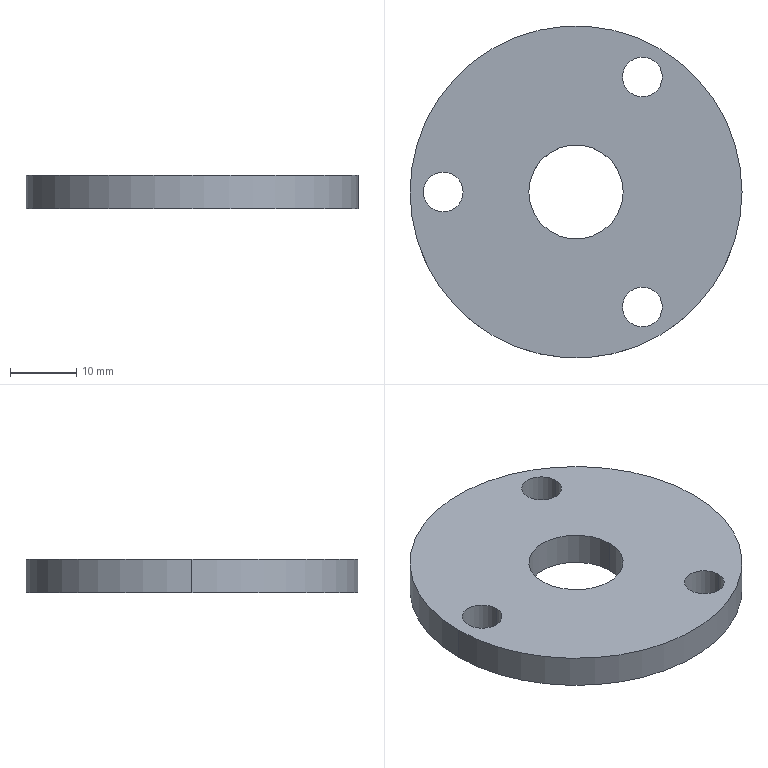Part | STEP file | 1 solid | 12 faces | box 50 x 50 x 5 mm | volume 8602 mm3 | cylinder 10 | plane 2 | commonest cylinder face diameters 6 x6 14.2 x2 50 x2
STEP:
#1=CARTESIAN_POINT('',(0.,0.,0.));
#2=DIRECTION('',(0.,0.,1.));
#3=DIRECTION('',(1.,0.,0.));
#4=AXIS2_PLACEMENT_3D('',#1,#2,#3);
#5=CARTESIAN_POINT('',(13.,17.321,0.));
#6=VERTEX_POINT('',#5);
#7=CARTESIAN_POINT('',(13.,17.321,5.));
#8=VERTEX_POINT('',#7);
#9=CARTESIAN_POINT('',(13.,17.321,15.));
#10=DIRECTION('',(0.,0.,1.));
#11=VECTOR('',#10,1.);
#12=LINE('',#9,#11);
#13=CARTESIAN_POINT('',(10.,17.321,15.));
#14=DIRECTION('',(0.,0.,1.));
#15=DIRECTION('',(1.,0.,0.));
#16=AXIS2_PLACEMENT_3D('',#13,#14,#15);
#17=CYLINDRICAL_SURFACE('',#16,3.);
#18=CARTESIAN_POINT('',(6.283,0.));
#19=DIRECTION('',(0.,1.));
#20=VECTOR('',#19,1.);
#21=LINE('',#18,#20);
#22=(GEOMETRIC_REPRESENTATION_CONTEXT(2)PARAMETRIC_REPRESENTATION_CONTEXT()REPRESENTATION_CONTEXT('',''));
#23=DEFINITIONAL_REPRESENTATION('',(#21),#22);
#24=PCURVE('',#17,#23);
#25=CARTESIAN_POINT('',(10.,17.321,15.));
#26=DIRECTION('',(0.,0.,1.));
#27=DIRECTION('',(1.,0.,0.));
#28=AXIS2_PLACEMENT_3D('',#25,#26,#27);
#29=CYLINDRICAL_SURFACE('',#28,3.);
#30=CARTESIAN_POINT('',(0.,0.));
#31=DIRECTION('',(0.,1.));
#32=VECTOR('',#31,1.);
#33=LINE('',#30,#32);
#34=(GEOMETRIC_REPRESENTATION_CONTEXT(2)PARAMETRIC_REPRESENTATION_CONTEXT()REPRESENTATION_CONTEXT('',''));
#35=DEFINITIONAL_REPRESENTATION('',(#33),#34);
#36=PCURVE('',#29,#35);
#37=SURFACE_CURVE('',#12,(#24,#36),.PCURVE_S1.);
#38=EDGE_CURVE('',#6,#8,#37,.T.);
#39=ORIENTED_EDGE('',*,*,#38,.T.);
#40=CARTESIAN_POINT('',(7.,17.321,5.));
#41=VERTEX_POINT('',#40);
#42=CARTESIAN_POINT('',(10.,17.321,5.));
#43=DIRECTION('',(0.,0.,-1.));
#44=DIRECTION('',(1.,0.,0.));
#45=AXIS2_PLACEMENT_3D('',#42,#43,#44);
#46=CIRCLE('',#45,3.);
#47=CARTESIAN_POINT('',(6.283,-10.));
#48=DIRECTION('',(-1.,0.));
#49=VECTOR('',#48,1.);
#50=LINE('',#47,#49);
#51=(GEOMETRIC_REPRESENTATION_CONTEXT(2)PARAMETRIC_REPRESENTATION_CONTEXT()REPRESENTATION_CONTEXT('',''));
#52=DEFINITIONAL_REPRESENTATION('',(#50),#51);
#53=PCURVE('',#17,#52);
#54=CARTESIAN_POINT('',(0.,0.,5.));
#55=DIRECTION('',(0.,0.,1.));
#56=DIRECTION('',(1.,0.,0.));
#57=AXIS2_PLACEMENT_3D('',#54,#55,#56);
#58=PLANE('',#57);
#59=CARTESIAN_POINT('',(13.,17.321));
#60=CARTESIAN_POINT('',(13.,12.124));
#61=CARTESIAN_POINT('',(8.5,14.722));
#62=CARTESIAN_POINT('',(4.,17.321));
#63=CARTESIAN_POINT('',(8.5,19.919));
#64=CARTESIAN_POINT('',(13.,22.517));
#65=CARTESIAN_POINT('',(13.,17.321));
#66=(BOUNDED_CURVE()B_SPLINE_CURVE(2,(#59,#60,#61,#62,#63,#64,#65),.UNSPECIFIED.,.T.,.F.)B_SPLINE_CURVE_WITH_KNOTS((1,2,2,2,2,1),(-2.094,0.,2.094,4.189,6.283,8.378),.UNSPECIFIED.)CURVE()GEOMETRIC_REPRESENTATION_ITEM()RATIONAL_B_SPLINE_CURVE((1.,0.5,1.,0.5,1.,0.5,1.))REPRESENTATION_ITEM(''));
#67=(GEOMETRIC_REPRESENTATION_CONTEXT(2)PARAMETRIC_REPRESENTATION_CONTEXT()REPRESENTATION_CONTEXT('',''));
#68=DEFINITIONAL_REPRESENTATION('',(#66),#67);
#69=PCURVE('',#58,#68);
#70=SURFACE_CURVE('',#46,(#53,#69),.PCURVE_S1.);
#71=EDGE_CURVE('',#8,#41,#70,.T.);
#72=ORIENTED_EDGE('',*,*,#71,.T.);
#73=CARTESIAN_POINT('',(7.,17.321,0.));
#74=VERTEX_POINT('',#73);
#75=CARTESIAN_POINT('',(7.,17.321,15.));
#76=DIRECTION('',(0.,0.,1.));
#77=VECTOR('',#76,1.);
#78=LINE('',#75,#77);
#79=CARTESIAN_POINT('',(3.142,0.));
#80=DIRECTION('',(0.,1.));
#81=VECTOR('',#80,1.);
#82=LINE('',#79,#81);
#83=(GEOMETRIC_REPRESENTATION_CONTEXT(2)PARAMETRIC_REPRESENTATION_CONTEXT()REPRESENTATION_CONTEXT('',''));
#84=DEFINITIONAL_REPRESENTATION('',(#82),#83);
#85=PCURVE('',#17,#84);
#86=CARTESIAN_POINT('',(3.142,0.));
#87=DIRECTION('',(0.,1.));
#88=VECTOR('',#87,1.);
#89=LINE('',#86,#88);
#90=(GEOMETRIC_REPRESENTATION_CONTEXT(2)PARAMETRIC_REPRESENTATION_CONTEXT()REPRESENTATION_CONTEXT('',''));
#91=DEFINITIONAL_REPRESENTATION('',(#89),#90);
#92=PCURVE('',#29,#91);
#93=SURFACE_CURVE('',#78,(#85,#92),.PCURVE_S1.);
#94=EDGE_CURVE('',#74,#41,#93,.T.);
#95=ORIENTED_EDGE('',*,*,#94,.F.);
#96=CARTESIAN_POINT('',(10.,17.321,0.));
#97=DIRECTION('',(0.,0.,1.));
#98=DIRECTION('',(1.,0.,0.));
#99=AXIS2_PLACEMENT_3D('',#96,#97,#98);
#100=CIRCLE('',#99,3.);
#101=CARTESIAN_POINT('',(0.,-15.));
#102=DIRECTION('',(1.,0.));
#103=VECTOR('',#102,1.);
#104=LINE('',#101,#103);
#105=(GEOMETRIC_REPRESENTATION_CONTEXT(2)PARAMETRIC_REPRESENTATION_CONTEXT()REPRESENTATION_CONTEXT('',''));
#106=DEFINITIONAL_REPRESENTATION('',(#104),#105);
#107=PCURVE('',#17,#106);
#108=CARTESIAN_POINT('',(0.,0.,0.));
#109=DIRECTION('',(0.,0.,1.));
#110=DIRECTION('',(1.,0.,0.));
#111=AXIS2_PLACEMENT_3D('',#108,#109,#110);
#112=PLANE('',#111);
#113=CARTESIAN_POINT('',(10.,17.321));
#114=DIRECTION('',(1.,0.));
#115=AXIS2_PLACEMENT_2D('',#113,#114);
#116=CIRCLE('',#115,3.);
#117=(GEOMETRIC_REPRESENTATION_CONTEXT(2)PARAMETRIC_REPRESENTATION_CONTEXT()REPRESENTATION_CONTEXT('',''));
#118=DEFINITIONAL_REPRESENTATION('',(#116),#117);
#119=PCURVE('',#112,#118);
#120=SURFACE_CURVE('',#100,(#107,#119),.PCURVE_S1.);
#121=EDGE_CURVE('',#74,#6,#120,.T.);
#122=ORIENTED_EDGE('',*,*,#121,.T.);
#123=EDGE_LOOP('',(#39,#72,#95,#122));
#124=FACE_BOUND('',#123,.F.);
#125=ADVANCED_FACE('',(#124),#17,.F.);
#126=CARTESIAN_POINT('',(7.1,0.,0.));
#127=VERTEX_POINT('',#126);
#128=CARTESIAN_POINT('',(7.1,0.,5.));
#129=VERTEX_POINT('',#128);
#130=CARTESIAN_POINT('',(7.1,0.,5.));
#131=DIRECTION('',(0.,0.,1.));
#132=VECTOR('',#131,1.);
#133=LINE('',#130,#132);
#134=CARTESIAN_POINT('',(0.,0.,5.));
#135=DIRECTION('',(0.,0.,1.));
#136=DIRECTION('',(1.,0.,0.));
#137=AXIS2_PLACEMENT_3D('',#134,#135,#136);
#138=CYLINDRICAL_SURFACE('',#137,7.1);
#139=CARTESIAN_POINT('',(6.283,0.));
#140=DIRECTION('',(0.,1.));
#141=VECTOR('',#140,1.);
#142=LINE('',#139,#141);
#143=(GEOMETRIC_REPRESENTATION_CONTEXT(2)PARAMETRIC_REPRESENTATION_CONTEXT()REPRESENTATION_CONTEXT('',''));
#144=DEFINITIONAL_REPRESENTATION('',(#142),#143);
#145=PCURVE('',#138,#144);
#146=CARTESIAN_POINT('',(0.,0.,5.));
#147=DIRECTION('',(0.,0.,1.));
#148=DIRECTION('',(1.,0.,0.));
#149=AXIS2_PLACEMENT_3D('',#146,#147,#148);
#150=CYLINDRICAL_SURFACE('',#149,7.1);
#151=CARTESIAN_POINT('',(0.,0.));
#152=DIRECTION('',(0.,1.));
#153=VECTOR('',#152,1.);
#154=LINE('',#151,#153);
#155=(GEOMETRIC_REPRESENTATION_CONTEXT(2)PARAMETRIC_REPRESENTATION_CONTEXT()REPRESENTATION_CONTEXT('',''));
#156=DEFINITIONAL_REPRESENTATION('',(#154),#155);
#157=PCURVE('',#150,#156);
#158=SURFACE_CURVE('',#133,(#145,#157),.PCURVE_S1.);
#159=EDGE_CURVE('',#127,#129,#158,.T.);
#160=ORIENTED_EDGE('',*,*,#159,.T.);
#161=CARTESIAN_POINT('',(-7.1,0.,5.));
#162=VERTEX_POINT('',#161);
#163=CARTESIAN_POINT('',(0.,0.,5.));
#164=DIRECTION('',(0.,0.,-1.));
#165=DIRECTION('',(1.,0.,0.));
#166=AXIS2_PLACEMENT_3D('',#163,#164,#165);
#167=CIRCLE('',#166,7.1);
#168=CARTESIAN_POINT('',(6.283,0.));
#169=DIRECTION('',(-1.,0.));
#170=VECTOR('',#169,1.);
#171=LINE('',#168,#170);
#172=(GEOMETRIC_REPRESENTATION_CONTEXT(2)PARAMETRIC_REPRESENTATION_CONTEXT()REPRESENTATION_CONTEXT('',''));
#173=DEFINITIONAL_REPRESENTATION('',(#171),#172);
#174=PCURVE('',#138,#173);
#175=CARTESIAN_POINT('',(7.1,0.));
#176=CARTESIAN_POINT('',(7.1,-12.298));
#177=CARTESIAN_POINT('',(-3.55,-6.149));
#178=CARTESIAN_POINT('',(-14.2,0.));
#179=CARTESIAN_POINT('',(-3.55,6.149));
#180=CARTESIAN_POINT('',(7.1,12.298));
#181=CARTESIAN_POINT('',(7.1,0.));
#182=(BOUNDED_CURVE()B_SPLINE_CURVE(2,(#175,#176,#177,#178,#179,#180,#181),.UNSPECIFIED.,.T.,.F.)B_SPLINE_CURVE_WITH_KNOTS((1,2,2,2,2,1),(-2.094,0.,2.094,4.189,6.283,8.378),.UNSPECIFIED.)CURVE()GEOMETRIC_REPRESENTATION_ITEM()RATIONAL_B_SPLINE_CURVE((1.,0.5,1.,0.5,1.,0.5,1.))REPRESENTATION_ITEM(''));
#183=(GEOMETRIC_REPRESENTATION_CONTEXT(2)PARAMETRIC_REPRESENTATION_CONTEXT()REPRESENTATION_CONTEXT('',''));
#184=DEFINITIONAL_REPRESENTATION('',(#182),#183);
#185=PCURVE('',#58,#184);
#186=SURFACE_CURVE('',#167,(#174,#185),.PCURVE_S1.);
#187=EDGE_CURVE('',#129,#162,#186,.T.);
#188=ORIENTED_EDGE('',*,*,#187,.T.);
#189=CARTESIAN_POINT('',(-7.1,0.,0.));
#190=VERTEX_POINT('',#189);
#191=CARTESIAN_POINT('',(-7.1,0.,5.));
#192=DIRECTION('',(0.,0.,1.));
#193=VECTOR('',#192,1.);
#194=LINE('',#191,#193);
#195=CARTESIAN_POINT('',(3.142,0.));
#196=DIRECTION('',(0.,1.));
#197=VECTOR('',#196,1.);
#198=LINE('',#195,#197);
#199=(GEOMETRIC_REPRESENTATION_CONTEXT(2)PARAMETRIC_REPRESENTATION_CONTEXT()REPRESENTATION_CONTEXT('',''));
#200=DEFINITIONAL_REPRESENTATION('',(#198),#199);
#201=PCURVE('',#138,#200);
#202=CARTESIAN_POINT('',(3.142,0.));
#203=DIRECTION('',(0.,1.));
#204=VECTOR('',#203,1.);
#205=LINE('',#202,#204);
#206=(GEOMETRIC_REPRESENTATION_CONTEXT(2)PARAMETRIC_REPRESENTATION_CONTEXT()REPRESENTATION_CONTEXT('',''));
#207=DEFINITIONAL_REPRESENTATION('',(#205),#206);
#208=PCURVE('',#150,#207);
#209=SURFACE_CURVE('',#194,(#201,#208),.PCURVE_S1.);
#210=EDGE_CURVE('',#190,#162,#209,.T.);
#211=ORIENTED_EDGE('',*,*,#210,.F.);
#212=CARTESIAN_POINT('',(0.,0.,0.));
#213=DIRECTION('',(0.,0.,1.));
#214=DIRECTION('',(1.,0.,0.));
#215=AXIS2_PLACEMENT_3D('',#212,#213,#214);
#216=CIRCLE('',#215,7.1);
#217=CARTESIAN_POINT('',(0.,-5.));
#218=DIRECTION('',(1.,0.));
#219=VECTOR('',#218,1.);
#220=LINE('',#217,#219);
#221=(GEOMETRIC_REPRESENTATION_CONTEXT(2)PARAMETRIC_REPRESENTATION_CONTEXT()REPRESENTATION_CONTEXT('',''));
#222=DEFINITIONAL_REPRESENTATION('',(#220),#221);
#223=PCURVE('',#138,#222);
#224=CARTESIAN_POINT('',(0.,0.));
#225=DIRECTION('',(1.,0.));
#226=AXIS2_PLACEMENT_2D('',#224,#225);
#227=CIRCLE('',#226,7.1);
#228=(GEOMETRIC_REPRESENTATION_CONTEXT(2)PARAMETRIC_REPRESENTATION_CONTEXT()REPRESENTATION_CONTEXT('',''));
#229=DEFINITIONAL_REPRESENTATION('',(#227),#228);
#230=PCURVE('',#112,#229);
#231=SURFACE_CURVE('',#216,(#223,#230),.PCURVE_S1.);
#232=EDGE_CURVE('',#190,#127,#231,.T.);
#233=ORIENTED_EDGE('',*,*,#232,.T.);
#234=EDGE_LOOP('',(#160,#188,#211,#233));
#235=FACE_BOUND('',#234,.F.);
#236=ADVANCED_FACE('',(#235),#138,.F.);
#237=CARTESIAN_POINT('',(-17.,0.,0.));
#238=VERTEX_POINT('',#237);
#239=CARTESIAN_POINT('',(-17.,0.,5.));
#240=VERTEX_POINT('',#239);
#241=CARTESIAN_POINT('',(-17.,0.,15.));
#242=DIRECTION('',(0.,0.,1.));
#243=VECTOR('',#242,1.);
#244=LINE('',#241,#243);
#245=CARTESIAN_POINT('',(-20.,0.,15.));
#246=DIRECTION('',(0.,0.,1.));
#247=DIRECTION('',(1.,0.,0.));
#248=AXIS2_PLACEMENT_3D('',#245,#246,#247);
#249=CYLINDRICAL_SURFACE('',#248,3.);
#250=CARTESIAN_POINT('',(6.283,0.));
#251=DIRECTION('',(0.,1.));
#252=VECTOR('',#251,1.);
#253=LINE('',#250,#252);
#254=(GEOMETRIC_REPRESENTATION_CONTEXT(2)PARAMETRIC_REPRESENTATION_CONTEXT()REPRESENTATION_CONTEXT('',''));
#255=DEFINITIONAL_REPRESENTATION('',(#253),#254);
#256=PCURVE('',#249,#255);
#257=CARTESIAN_POINT('',(-20.,0.,15.));
#258=DIRECTION('',(0.,0.,1.));
#259=DIRECTION('',(1.,0.,0.));
#260=AXIS2_PLACEMENT_3D('',#257,#258,#259);
#261=CYLINDRICAL_SURFACE('',#260,3.);
#262=CARTESIAN_POINT('',(0.,0.));
#263=DIRECTION('',(0.,1.));
#264=VECTOR('',#263,1.);
#265=LINE('',#262,#264);
#266=(GEOMETRIC_REPRESENTATION_CONTEXT(2)PARAMETRIC_REPRESENTATION_CONTEXT()REPRESENTATION_CONTEXT('',''));
#267=DEFINITIONAL_REPRESENTATION('',(#265),#266);
#268=PCURVE('',#261,#267);
#269=SURFACE_CURVE('',#244,(#256,#268),.PCURVE_S1.);
#270=EDGE_CURVE('',#238,#240,#269,.T.);
#271=ORIENTED_EDGE('',*,*,#270,.T.);
#272=CARTESIAN_POINT('',(-23.,0.,5.));
#273=VERTEX_POINT('',#272);
#274=CARTESIAN_POINT('',(-20.,0.,5.));
#275=DIRECTION('',(0.,0.,-1.));
#276=DIRECTION('',(1.,0.,0.));
#277=AXIS2_PLACEMENT_3D('',#274,#275,#276);
#278=CIRCLE('',#277,3.);
#279=CARTESIAN_POINT('',(6.283,-10.));
#280=DIRECTION('',(-1.,0.));
#281=VECTOR('',#280,1.);
#282=LINE('',#279,#281);
#283=(GEOMETRIC_REPRESENTATION_CONTEXT(2)PARAMETRIC_REPRESENTATION_CONTEXT()REPRESENTATION_CONTEXT('',''));
#284=DEFINITIONAL_REPRESENTATION('',(#282),#283);
#285=PCURVE('',#249,#284);
#286=CARTESIAN_POINT('',(-17.,0.));
#287=CARTESIAN_POINT('',(-17.,-5.196));
#288=CARTESIAN_POINT('',(-21.5,-2.598));
#289=CARTESIAN_POINT('',(-26.,0.));
#290=CARTESIAN_POINT('',(-21.5,2.598));
#291=CARTESIAN_POINT('',(-17.,5.196));
#292=CARTESIAN_POINT('',(-17.,0.));
#293=(BOUNDED_CURVE()B_SPLINE_CURVE(2,(#286,#287,#288,#289,#290,#291,#292),.UNSPECIFIED.,.T.,.F.)B_SPLINE_CURVE_WITH_KNOTS((1,2,2,2,2,1),(-2.094,0.,2.094,4.189,6.283,8.378),.UNSPECIFIED.)CURVE()GEOMETRIC_REPRESENTATION_ITEM()RATIONAL_B_SPLINE_CURVE((1.,0.5,1.,0.5,1.,0.5,1.))REPRESENTATION_ITEM(''));
#294=(GEOMETRIC_REPRESENTATION_CONTEXT(2)PARAMETRIC_REPRESENTATION_CONTEXT()REPRESENTATION_CONTEXT('',''));
#295=DEFINITIONAL_REPRESENTATION('',(#293),#294);
#296=PCURVE('',#58,#295);
#297=SURFACE_CURVE('',#278,(#285,#296),.PCURVE_S1.);
#298=EDGE_CURVE('',#240,#273,#297,.T.);
#299=ORIENTED_EDGE('',*,*,#298,.T.);
#300=CARTESIAN_POINT('',(-23.,0.,0.));
#301=VERTEX_POINT('',#300);
#302=CARTESIAN_POINT('',(-23.,0.,15.));
#303=DIRECTION('',(0.,0.,1.));
#304=VECTOR('',#303,1.);
#305=LINE('',#302,#304);
#306=CARTESIAN_POINT('',(3.142,0.));
#307=DIRECTION('',(0.,1.));
#308=VECTOR('',#307,1.);
#309=LINE('',#306,#308);
#310=(GEOMETRIC_REPRESENTATION_CONTEXT(2)PARAMETRIC_REPRESENTATION_CONTEXT()REPRESENTATION_CONTEXT('',''));
#311=DEFINITIONAL_REPRESENTATION('',(#309),#310);
#312=PCURVE('',#249,#311);
#313=CARTESIAN_POINT('',(3.142,0.));
#314=DIRECTION('',(0.,1.));
#315=VECTOR('',#314,1.);
#316=LINE('',#313,#315);
#317=(GEOMETRIC_REPRESENTATION_CONTEXT(2)PARAMETRIC_REPRESENTATION_CONTEXT()REPRESENTATION_CONTEXT('',''));
#318=DEFINITIONAL_REPRESENTATION('',(#316),#317);
#319=PCURVE('',#261,#318);
#320=SURFACE_CURVE('',#305,(#312,#319),.PCURVE_S1.);
#321=EDGE_CURVE('',#301,#273,#320,.T.);
#322=ORIENTED_EDGE('',*,*,#321,.F.);
#323=CARTESIAN_POINT('',(-20.,0.,0.));
#324=DIRECTION('',(0.,0.,1.));
#325=DIRECTION('',(1.,0.,0.));
#326=AXIS2_PLACEMENT_3D('',#323,#324,#325);
#327=CIRCLE('',#326,3.);
#328=CARTESIAN_POINT('',(0.,-15.));
#329=DIRECTION('',(1.,0.));
#330=VECTOR('',#329,1.);
#331=LINE('',#328,#330);
#332=(GEOMETRIC_REPRESENTATION_CONTEXT(2)PARAMETRIC_REPRESENTATION_CONTEXT()REPRESENTATION_CONTEXT('',''));
#333=DEFINITIONAL_REPRESENTATION('',(#331),#332);
#334=PCURVE('',#249,#333);
#335=CARTESIAN_POINT('',(-20.,0.));
#336=DIRECTION('',(1.,0.));
#337=AXIS2_PLACEMENT_2D('',#335,#336);
#338=CIRCLE('',#337,3.);
#339=(GEOMETRIC_REPRESENTATION_CONTEXT(2)PARAMETRIC_REPRESENTATION_CONTEXT()REPRESENTATION_CONTEXT('',''));
#340=DEFINITIONAL_REPRESENTATION('',(#338),#339);
#341=PCURVE('',#112,#340);
#342=SURFACE_CURVE('',#327,(#334,#341),.PCURVE_S1.);
#343=EDGE_CURVE('',#301,#238,#342,.T.);
#344=ORIENTED_EDGE('',*,*,#343,.T.);
#345=EDGE_LOOP('',(#271,#299,#322,#344));
#346=FACE_BOUND('',#345,.F.);
#347=ADVANCED_FACE('',(#346),#249,.F.);
#348=CARTESIAN_POINT('',(13.,-17.321,0.));
#349=VERTEX_POINT('',#348);
#350=CARTESIAN_POINT('',(13.,-17.321,5.));
#351=VERTEX_POINT('',#350);
#352=CARTESIAN_POINT('',(13.,-17.321,15.));
#353=DIRECTION('',(0.,0.,1.));
#354=VECTOR('',#353,1.);
#355=LINE('',#352,#354);
#356=CARTESIAN_POINT('',(10.,-17.321,15.));
#357=DIRECTION('',(0.,0.,1.));
#358=DIRECTION('',(1.,0.,0.));
#359=AXIS2_PLACEMENT_3D('',#356,#357,#358);
#360=CYLINDRICAL_SURFACE('',#359,3.);
#361=CARTESIAN_POINT('',(6.283,0.));
#362=DIRECTION('',(0.,1.));
#363=VECTOR('',#362,1.);
#364=LINE('',#361,#363);
#365=(GEOMETRIC_REPRESENTATION_CONTEXT(2)PARAMETRIC_REPRESENTATION_CONTEXT()REPRESENTATION_CONTEXT('',''));
#366=DEFINITIONAL_REPRESENTATION('',(#364),#365);
#367=PCURVE('',#360,#366);
#368=CARTESIAN_POINT('',(10.,-17.321,15.));
#369=DIRECTION('',(0.,0.,1.));
#370=DIRECTION('',(1.,0.,0.));
#371=AXIS2_PLACEMENT_3D('',#368,#369,#370);
#372=CYLINDRICAL_SURFACE('',#371,3.);
#373=CARTESIAN_POINT('',(0.,0.));
#374=DIRECTION('',(0.,1.));
#375=VECTOR('',#374,1.);
#376=LINE('',#373,#375);
#377=(GEOMETRIC_REPRESENTATION_CONTEXT(2)PARAMETRIC_REPRESENTATION_CONTEXT()REPRESENTATION_CONTEXT('',''));
#378=DEFINITIONAL_REPRESENTATION('',(#376),#377);
#379=PCURVE('',#372,#378);
#380=SURFACE_CURVE('',#355,(#367,#379),.PCURVE_S1.);
#381=EDGE_CURVE('',#349,#351,#380,.T.);
#382=ORIENTED_EDGE('',*,*,#381,.T.);
#383=CARTESIAN_POINT('',(7.,-17.321,5.));
#384=VERTEX_POINT('',#383);
#385=CARTESIAN_POINT('',(10.,-17.321,5.));
#386=DIRECTION('',(0.,0.,-1.));
#387=DIRECTION('',(1.,0.,0.));
#388=AXIS2_PLACEMENT_3D('',#385,#386,#387);
#389=CIRCLE('',#388,3.);
#390=CARTESIAN_POINT('',(6.283,-10.));
#391=DIRECTION('',(-1.,0.));
#392=VECTOR('',#391,1.);
#393=LINE('',#390,#392);
#394=(GEOMETRIC_REPRESENTATION_CONTEXT(2)PARAMETRIC_REPRESENTATION_CONTEXT()REPRESENTATION_CONTEXT('',''));
#395=DEFINITIONAL_REPRESENTATION('',(#393),#394);
#396=PCURVE('',#360,#395);
#397=CARTESIAN_POINT('',(13.,-17.321));
#398=CARTESIAN_POINT('',(13.,-22.517));
#399=CARTESIAN_POINT('',(8.5,-19.919));
#400=CARTESIAN_POINT('',(4.,-17.321));
#401=CARTESIAN_POINT('',(8.5,-14.722));
#402=CARTESIAN_POINT('',(13.,-12.124));
#403=CARTESIAN_POINT('',(13.,-17.321));
#404=(BOUNDED_CURVE()B_SPLINE_CURVE(2,(#397,#398,#399,#400,#401,#402,#403),.UNSPECIFIED.,.T.,.F.)B_SPLINE_CURVE_WITH_KNOTS((1,2,2,2,2,1),(-2.094,0.,2.094,4.189,6.283,8.378),.UNSPECIFIED.)CURVE()GEOMETRIC_REPRESENTATION_ITEM()RATIONAL_B_SPLINE_CURVE((1.,0.5,1.,0.5,1.,0.5,1.))REPRESENTATION_ITEM(''));
#405=(GEOMETRIC_REPRESENTATION_CONTEXT(2)PARAMETRIC_REPRESENTATION_CONTEXT()REPRESENTATION_CONTEXT('',''));
#406=DEFINITIONAL_REPRESENTATION('',(#404),#405);
#407=PCURVE('',#58,#406);
#408=SURFACE_CURVE('',#389,(#396,#407),.PCURVE_S1.);
#409=EDGE_CURVE('',#351,#384,#408,.T.);
#410=ORIENTED_EDGE('',*,*,#409,.T.);
#411=CARTESIAN_POINT('',(7.,-17.321,0.));
#412=VERTEX_POINT('',#411);
#413=CARTESIAN_POINT('',(7.,-17.321,15.));
#414=DIRECTION('',(0.,0.,1.));
#415=VECTOR('',#414,1.);
#416=LINE('',#413,#415);
#417=CARTESIAN_POINT('',(3.142,0.));
#418=DIRECTION('',(0.,1.));
#419=VECTOR('',#418,1.);
#420=LINE('',#417,#419);
#421=(GEOMETRIC_REPRESENTATION_CONTEXT(2)PARAMETRIC_REPRESENTATION_CONTEXT()REPRESENTATION_CONTEXT('',''));
#422=DEFINITIONAL_REPRESENTATION('',(#420),#421);
#423=PCURVE('',#360,#422);
#424=CARTESIAN_POINT('',(3.142,0.));
#425=DIRECTION('',(0.,1.));
#426=VECTOR('',#425,1.);
#427=LINE('',#424,#426);
#428=(GEOMETRIC_REPRESENTATION_CONTEXT(2)PARAMETRIC_REPRESENTATION_CONTEXT()REPRESENTATION_CONTEXT('',''));
#429=DEFINITIONAL_REPRESENTATION('',(#427),#428);
#430=PCURVE('',#372,#429);
#431=SURFACE_CURVE('',#416,(#423,#430),.PCURVE_S1.);
#432=EDGE_CURVE('',#412,#384,#431,.T.);
#433=ORIENTED_EDGE('',*,*,#432,.F.);
#434=CARTESIAN_POINT('',(10.,-17.321,0.));
#435=DIRECTION('',(0.,0.,1.));
#436=DIRECTION('',(1.,0.,0.));
#437=AXIS2_PLACEMENT_3D('',#434,#435,#436);
#438=CIRCLE('',#437,3.);
#439=CARTESIAN_POINT('',(0.,-15.));
#440=DIRECTION('',(1.,0.));
#441=VECTOR('',#440,1.);
#442=LINE('',#439,#441);
#443=(GEOMETRIC_REPRESENTATION_CONTEXT(2)PARAMETRIC_REPRESENTATION_CONTEXT()REPRESENTATION_CONTEXT('',''));
#444=DEFINITIONAL_REPRESENTATION('',(#442),#443);
#445=PCURVE('',#360,#444);
#446=CARTESIAN_POINT('',(10.,-17.321));
#447=DIRECTION('',(1.,0.));
#448=AXIS2_PLACEMENT_2D('',#446,#447);
#449=CIRCLE('',#448,3.);
#450=(GEOMETRIC_REPRESENTATION_CONTEXT(2)PARAMETRIC_REPRESENTATION_CONTEXT()REPRESENTATION_CONTEXT('',''));
#451=DEFINITIONAL_REPRESENTATION('',(#449),#450);
#452=PCURVE('',#112,#451);
#453=SURFACE_CURVE('',#438,(#445,#452),.PCURVE_S1.);
#454=EDGE_CURVE('',#412,#349,#453,.T.);
#455=ORIENTED_EDGE('',*,*,#454,.T.);
#456=EDGE_LOOP('',(#382,#410,#433,#455));
#457=FACE_BOUND('',#456,.F.);
#458=ADVANCED_FACE('',(#457),#360,.F.);
#459=CARTESIAN_POINT('',(25.,0.,0.));
#460=VERTEX_POINT('',#459);
#461=CARTESIAN_POINT('',(-25.,0.,0.));
#462=VERTEX_POINT('',#461);
#463=CARTESIAN_POINT('',(0.,0.,0.));
#464=DIRECTION('',(0.,0.,1.));
#465=DIRECTION('',(1.,0.,0.));
#466=AXIS2_PLACEMENT_3D('',#463,#464,#465);
#467=CIRCLE('',#466,25.);
#468=CARTESIAN_POINT('',(0.,0.,5.));
#469=DIRECTION('',(0.,0.,1.));
#470=DIRECTION('',(1.,0.,0.));
#471=AXIS2_PLACEMENT_3D('',#468,#469,#470);
#472=CYLINDRICAL_SURFACE('',#471,25.);
#473=CARTESIAN_POINT('',(0.,-5.));
#474=DIRECTION('',(1.,0.));
#475=VECTOR('',#474,1.);
#476=LINE('',#473,#475);
#477=(GEOMETRIC_REPRESENTATION_CONTEXT(2)PARAMETRIC_REPRESENTATION_CONTEXT()REPRESENTATION_CONTEXT('',''));
#478=DEFINITIONAL_REPRESENTATION('',(#476),#477);
#479=PCURVE('',#472,#478);
#480=CARTESIAN_POINT('',(0.,0.));
#481=DIRECTION('',(1.,0.));
#482=AXIS2_PLACEMENT_2D('',#480,#481);
#483=CIRCLE('',#482,25.);
#484=(GEOMETRIC_REPRESENTATION_CONTEXT(2)PARAMETRIC_REPRESENTATION_CONTEXT()REPRESENTATION_CONTEXT('',''));
#485=DEFINITIONAL_REPRESENTATION('',(#483),#484);
#486=PCURVE('',#112,#485);
#487=SURFACE_CURVE('',#467,(#479,#486),.PCURVE_S1.);
#488=EDGE_CURVE('',#460,#462,#487,.T.);
#489=ORIENTED_EDGE('',*,*,#488,.T.);
#490=CARTESIAN_POINT('',(-25.,0.,5.));
#491=VERTEX_POINT('',#490);
#492=CARTESIAN_POINT('',(-25.,0.,5.));
#493=DIRECTION('',(0.,0.,1.));
#494=VECTOR('',#493,1.);
#495=LINE('',#492,#494);
#496=CARTESIAN_POINT('',(3.142,0.));
#497=DIRECTION('',(0.,1.));
#498=VECTOR('',#497,1.);
#499=LINE('',#496,#498);
#500=(GEOMETRIC_REPRESENTATION_CONTEXT(2)PARAMETRIC_REPRESENTATION_CONTEXT()REPRESENTATION_CONTEXT('',''));
#501=DEFINITIONAL_REPRESENTATION('',(#499),#500);
#502=PCURVE('',#472,#501);
#503=CARTESIAN_POINT('',(0.,0.,5.));
#504=DIRECTION('',(0.,0.,1.));
#505=DIRECTION('',(1.,0.,0.));
#506=AXIS2_PLACEMENT_3D('',#503,#504,#505);
#507=CYLINDRICAL_SURFACE('',#506,25.);
#508=CARTESIAN_POINT('',(3.142,0.));
#509=DIRECTION('',(0.,1.));
#510=VECTOR('',#509,1.);
#511=LINE('',#508,#510);
#512=(GEOMETRIC_REPRESENTATION_CONTEXT(2)PARAMETRIC_REPRESENTATION_CONTEXT()REPRESENTATION_CONTEXT('',''));
#513=DEFINITIONAL_REPRESENTATION('',(#511),#512);
#514=PCURVE('',#507,#513);
#515=SURFACE_CURVE('',#495,(#502,#514),.PCURVE_S1.);
#516=EDGE_CURVE('',#462,#491,#515,.T.);
#517=ORIENTED_EDGE('',*,*,#516,.T.);
#518=CARTESIAN_POINT('',(25.,0.,5.));
#519=VERTEX_POINT('',#518);
#520=CARTESIAN_POINT('',(0.,0.,5.));
#521=DIRECTION('',(0.,0.,1.));
#522=DIRECTION('',(1.,0.,0.));
#523=AXIS2_PLACEMENT_3D('',#520,#521,#522);
#524=CIRCLE('',#523,25.);
#525=CARTESIAN_POINT('',(0.,0.));
#526=DIRECTION('',(1.,0.));
#527=VECTOR('',#526,1.);
#528=LINE('',#525,#527);
#529=(GEOMETRIC_REPRESENTATION_CONTEXT(2)PARAMETRIC_REPRESENTATION_CONTEXT()REPRESENTATION_CONTEXT('',''));
#530=DEFINITIONAL_REPRESENTATION('',(#528),#529);
#531=PCURVE('',#472,#530);
#532=CARTESIAN_POINT('',(0.,0.));
#533=DIRECTION('',(1.,0.));
#534=AXIS2_PLACEMENT_2D('',#532,#533);
#535=CIRCLE('',#534,25.);
#536=(GEOMETRIC_REPRESENTATION_CONTEXT(2)PARAMETRIC_REPRESENTATION_CONTEXT()REPRESENTATION_CONTEXT('',''));
#537=DEFINITIONAL_REPRESENTATION('',(#535),#536);
#538=PCURVE('',#58,#537);
#539=SURFACE_CURVE('',#524,(#531,#538),.PCURVE_S1.);
#540=EDGE_CURVE('',#519,#491,#539,.T.);
#541=ORIENTED_EDGE('',*,*,#540,.F.);
#542=CARTESIAN_POINT('',(25.,0.,5.));
#543=DIRECTION('',(0.,0.,1.));
#544=VECTOR('',#543,1.);
#545=LINE('',#542,#544);
#546=CARTESIAN_POINT('',(0.,0.));
#547=DIRECTION('',(0.,1.));
#548=VECTOR('',#547,1.);
#549=LINE('',#546,#548);
#550=(GEOMETRIC_REPRESENTATION_CONTEXT(2)PARAMETRIC_REPRESENTATION_CONTEXT()REPRESENTATION_CONTEXT('',''));
#551=DEFINITIONAL_REPRESENTATION('',(#549),#550);
#552=PCURVE('',#472,#551);
#553=CARTESIAN_POINT('',(6.283,0.));
#554=DIRECTION('',(0.,1.));
#555=VECTOR('',#554,1.);
#556=LINE('',#553,#555);
#557=(GEOMETRIC_REPRESENTATION_CONTEXT(2)PARAMETRIC_REPRESENTATION_CONTEXT()REPRESENTATION_CONTEXT('',''));
#558=DEFINITIONAL_REPRESENTATION('',(#556),#557);
#559=PCURVE('',#507,#558);
#560=SURFACE_CURVE('',#545,(#552,#559),.PCURVE_S1.);
#561=EDGE_CURVE('',#460,#519,#560,.T.);
#562=ORIENTED_EDGE('',*,*,#561,.F.);
#563=EDGE_LOOP('',(#489,#517,#541,#562));
#564=FACE_BOUND('',#563,.T.);
#565=ADVANCED_FACE('',(#564),#472,.T.);
#566=ORIENTED_EDGE('',*,*,#71,.T.);
#567=CARTESIAN_POINT('',(10.,17.321,5.));
#568=DIRECTION('',(0.,0.,-1.));
#569=DIRECTION('',(1.,0.,0.));
#570=AXIS2_PLACEMENT_3D('',#567,#568,#569);
#571=CIRCLE('',#570,3.);
#572=CARTESIAN_POINT('',(13.,17.321));
#573=CARTESIAN_POINT('',(13.,12.124));
#574=CARTESIAN_POINT('',(8.5,14.722));
#575=CARTESIAN_POINT('',(4.,17.321));
#576=CARTESIAN_POINT('',(8.5,19.919));
#577=CARTESIAN_POINT('',(13.,22.517));
#578=CARTESIAN_POINT('',(13.,17.321));
#579=(BOUNDED_CURVE()B_SPLINE_CURVE(2,(#572,#573,#574,#575,#576,#577,#578),.UNSPECIFIED.,.T.,.F.)B_SPLINE_CURVE_WITH_KNOTS((1,2,2,2,2,1),(-2.094,0.,2.094,4.189,6.283,8.378),.UNSPECIFIED.)CURVE()GEOMETRIC_REPRESENTATION_ITEM()RATIONAL_B_SPLINE_CURVE((1.,0.5,1.,0.5,1.,0.5,1.))REPRESENTATION_ITEM(''));
#580=(GEOMETRIC_REPRESENTATION_CONTEXT(2)PARAMETRIC_REPRESENTATION_CONTEXT()REPRESENTATION_CONTEXT('',''));
#581=DEFINITIONAL_REPRESENTATION('',(#579),#580);
#582=PCURVE('',#58,#581);
#583=CARTESIAN_POINT('',(6.283,-10.));
#584=DIRECTION('',(-1.,0.));
#585=VECTOR('',#584,1.);
#586=LINE('',#583,#585);
#587=(GEOMETRIC_REPRESENTATION_CONTEXT(2)PARAMETRIC_REPRESENTATION_CONTEXT()REPRESENTATION_CONTEXT('',''));
#588=DEFINITIONAL_REPRESENTATION('',(#586),#587);
#589=PCURVE('',#29,#588);
#590=SURFACE_CURVE('',#571,(#582,#589),.PCURVE_S1.);
#591=EDGE_CURVE('',#41,#8,#590,.T.);
#592=ORIENTED_EDGE('',*,*,#591,.T.);
#593=EDGE_LOOP('',(#566,#592));
#594=FACE_BOUND('',#593,.T.);
#595=ORIENTED_EDGE('',*,*,#187,.T.);
#596=CARTESIAN_POINT('',(0.,0.,5.));
#597=DIRECTION('',(0.,0.,-1.));
#598=DIRECTION('',(1.,0.,0.));
#599=AXIS2_PLACEMENT_3D('',#596,#597,#598);
#600=CIRCLE('',#599,7.1);
#601=CARTESIAN_POINT('',(7.1,0.));
#602=CARTESIAN_POINT('',(7.1,-12.298));
#603=CARTESIAN_POINT('',(-3.55,-6.149));
#604=CARTESIAN_POINT('',(-14.2,0.));
#605=CARTESIAN_POINT('',(-3.55,6.149));
#606=CARTESIAN_POINT('',(7.1,12.298));
#607=CARTESIAN_POINT('',(7.1,0.));
#608=(BOUNDED_CURVE()B_SPLINE_CURVE(2,(#601,#602,#603,#604,#605,#606,#607),.UNSPECIFIED.,.T.,.F.)B_SPLINE_CURVE_WITH_KNOTS((1,2,2,2,2,1),(-2.094,0.,2.094,4.189,6.283,8.378),.UNSPECIFIED.)CURVE()GEOMETRIC_REPRESENTATION_ITEM()RATIONAL_B_SPLINE_CURVE((1.,0.5,1.,0.5,1.,0.5,1.))REPRESENTATION_ITEM(''));
#609=(GEOMETRIC_REPRESENTATION_CONTEXT(2)PARAMETRIC_REPRESENTATION_CONTEXT()REPRESENTATION_CONTEXT('',''));
#610=DEFINITIONAL_REPRESENTATION('',(#608),#609);
#611=PCURVE('',#58,#610);
#612=CARTESIAN_POINT('',(6.283,0.));
#613=DIRECTION('',(-1.,0.));
#614=VECTOR('',#613,1.);
#615=LINE('',#612,#614);
#616=(GEOMETRIC_REPRESENTATION_CONTEXT(2)PARAMETRIC_REPRESENTATION_CONTEXT()REPRESENTATION_CONTEXT('',''));
#617=DEFINITIONAL_REPRESENTATION('',(#615),#616);
#618=PCURVE('',#150,#617);
#619=SURFACE_CURVE('',#600,(#611,#618),.PCURVE_S1.);
#620=EDGE_CURVE('',#162,#129,#619,.T.);
#621=ORIENTED_EDGE('',*,*,#620,.T.);
#622=EDGE_LOOP('',(#595,#621));
#623=FACE_BOUND('',#622,.T.);
#624=ORIENTED_EDGE('',*,*,#298,.T.);
#625=CARTESIAN_POINT('',(-20.,0.,5.));
#626=DIRECTION('',(0.,0.,-1.));
#627=DIRECTION('',(1.,0.,0.));
#628=AXIS2_PLACEMENT_3D('',#625,#626,#627);
#629=CIRCLE('',#628,3.);
#630=CARTESIAN_POINT('',(-17.,0.));
#631=CARTESIAN_POINT('',(-17.,-5.196));
#632=CARTESIAN_POINT('',(-21.5,-2.598));
#633=CARTESIAN_POINT('',(-26.,0.));
#634=CARTESIAN_POINT('',(-21.5,2.598));
#635=CARTESIAN_POINT('',(-17.,5.196));
#636=CARTESIAN_POINT('',(-17.,0.));
#637=(BOUNDED_CURVE()B_SPLINE_CURVE(2,(#630,#631,#632,#633,#634,#635,#636),.UNSPECIFIED.,.T.,.F.)B_SPLINE_CURVE_WITH_KNOTS((1,2,2,2,2,1),(-2.094,0.,2.094,4.189,6.283,8.378),.UNSPECIFIED.)CURVE()GEOMETRIC_REPRESENTATION_ITEM()RATIONAL_B_SPLINE_CURVE((1.,0.5,1.,0.5,1.,0.5,1.))REPRESENTATION_ITEM(''));
#638=(GEOMETRIC_REPRESENTATION_CONTEXT(2)PARAMETRIC_REPRESENTATION_CONTEXT()REPRESENTATION_CONTEXT('',''));
#639=DEFINITIONAL_REPRESENTATION('',(#637),#638);
#640=PCURVE('',#58,#639);
#641=CARTESIAN_POINT('',(6.283,-10.));
#642=DIRECTION('',(-1.,0.));
#643=VECTOR('',#642,1.);
#644=LINE('',#641,#643);
#645=(GEOMETRIC_REPRESENTATION_CONTEXT(2)PARAMETRIC_REPRESENTATION_CONTEXT()REPRESENTATION_CONTEXT('',''));
#646=DEFINITIONAL_REPRESENTATION('',(#644),#645);
#647=PCURVE('',#261,#646);
#648=SURFACE_CURVE('',#629,(#640,#647),.PCURVE_S1.);
#649=EDGE_CURVE('',#273,#240,#648,.T.);
#650=ORIENTED_EDGE('',*,*,#649,.T.);
#651=EDGE_LOOP('',(#624,#650));
#652=FACE_BOUND('',#651,.T.);
#653=ORIENTED_EDGE('',*,*,#409,.T.);
#654=CARTESIAN_POINT('',(10.,-17.321,5.));
#655=DIRECTION('',(0.,0.,-1.));
#656=DIRECTION('',(1.,0.,0.));
#657=AXIS2_PLACEMENT_3D('',#654,#655,#656);
#658=CIRCLE('',#657,3.);
#659=CARTESIAN_POINT('',(13.,-17.321));
#660=CARTESIAN_POINT('',(13.,-22.517));
#661=CARTESIAN_POINT('',(8.5,-19.919));
#662=CARTESIAN_POINT('',(4.,-17.321));
#663=CARTESIAN_POINT('',(8.5,-14.722));
#664=CARTESIAN_POINT('',(13.,-12.124));
#665=CARTESIAN_POINT('',(13.,-17.321));
#666=(BOUNDED_CURVE()B_SPLINE_CURVE(2,(#659,#660,#661,#662,#663,#664,#665),.UNSPECIFIED.,.T.,.F.)B_SPLINE_CURVE_WITH_KNOTS((1,2,2,2,2,1),(-2.094,0.,2.094,4.189,6.283,8.378),.UNSPECIFIED.)CURVE()GEOMETRIC_REPRESENTATION_ITEM()RATIONAL_B_SPLINE_CURVE((1.,0.5,1.,0.5,1.,0.5,1.))REPRESENTATION_ITEM(''));
#667=(GEOMETRIC_REPRESENTATION_CONTEXT(2)PARAMETRIC_REPRESENTATION_CONTEXT()REPRESENTATION_CONTEXT('',''));
#668=DEFINITIONAL_REPRESENTATION('',(#666),#667);
#669=PCURVE('',#58,#668);
#670=CARTESIAN_POINT('',(6.283,-10.));
#671=DIRECTION('',(-1.,0.));
#672=VECTOR('',#671,1.);
#673=LINE('',#670,#672);
#674=(GEOMETRIC_REPRESENTATION_CONTEXT(2)PARAMETRIC_REPRESENTATION_CONTEXT()REPRESENTATION_CONTEXT('',''));
#675=DEFINITIONAL_REPRESENTATION('',(#673),#674);
#676=PCURVE('',#372,#675);
#677=SURFACE_CURVE('',#658,(#669,#676),.PCURVE_S1.);
#678=EDGE_CURVE('',#384,#351,#677,.T.);
#679=ORIENTED_EDGE('',*,*,#678,.T.);
#680=EDGE_LOOP('',(#653,#679));
#681=FACE_BOUND('',#680,.T.);
#682=ORIENTED_EDGE('',*,*,#540,.T.);
#683=CARTESIAN_POINT('',(0.,0.,5.));
#684=DIRECTION('',(0.,0.,1.));
#685=DIRECTION('',(1.,0.,0.));
#686=AXIS2_PLACEMENT_3D('',#683,#684,#685);
#687=CIRCLE('',#686,25.);
#688=CARTESIAN_POINT('',(0.,0.));
#689=DIRECTION('',(1.,0.));
#690=AXIS2_PLACEMENT_2D('',#688,#689);
#691=CIRCLE('',#690,25.);
#692=(GEOMETRIC_REPRESENTATION_CONTEXT(2)PARAMETRIC_REPRESENTATION_CONTEXT()REPRESENTATION_CONTEXT('',''));
#693=DEFINITIONAL_REPRESENTATION('',(#691),#692);
#694=PCURVE('',#58,#693);
#695=CARTESIAN_POINT('',(0.,0.));
#696=DIRECTION('',(1.,0.));
#697=VECTOR('',#696,1.);
#698=LINE('',#695,#697);
#699=(GEOMETRIC_REPRESENTATION_CONTEXT(2)PARAMETRIC_REPRESENTATION_CONTEXT()REPRESENTATION_CONTEXT('',''));
#700=DEFINITIONAL_REPRESENTATION('',(#698),#699);
#701=PCURVE('',#507,#700);
#702=SURFACE_CURVE('',#687,(#694,#701),.PCURVE_S1.);
#703=EDGE_CURVE('',#491,#519,#702,.T.);
#704=ORIENTED_EDGE('',*,*,#703,.T.);
#705=EDGE_LOOP('',(#682,#704));
#706=FACE_BOUND('',#705,.T.);
#707=ADVANCED_FACE('',(#594,#623,#652,#681,#706),#58,.T.);
#708=ORIENTED_EDGE('',*,*,#591,.T.);
#709=ORIENTED_EDGE('',*,*,#38,.F.);
#710=CARTESIAN_POINT('',(10.,17.321,0.));
#711=DIRECTION('',(0.,0.,1.));
#712=DIRECTION('',(1.,0.,0.));
#713=AXIS2_PLACEMENT_3D('',#710,#711,#712);
#714=CIRCLE('',#713,3.);
#715=CARTESIAN_POINT('',(0.,-15.));
#716=DIRECTION('',(1.,0.));
#717=VECTOR('',#716,1.);
#718=LINE('',#715,#717);
#719=(GEOMETRIC_REPRESENTATION_CONTEXT(2)PARAMETRIC_REPRESENTATION_CONTEXT()REPRESENTATION_CONTEXT('',''));
#720=DEFINITIONAL_REPRESENTATION('',(#718),#719);
#721=PCURVE('',#29,#720);
#722=CARTESIAN_POINT('',(10.,17.321));
#723=DIRECTION('',(1.,0.));
#724=AXIS2_PLACEMENT_2D('',#722,#723);
#725=CIRCLE('',#724,3.);
#726=(GEOMETRIC_REPRESENTATION_CONTEXT(2)PARAMETRIC_REPRESENTATION_CONTEXT()REPRESENTATION_CONTEXT('',''));
#727=DEFINITIONAL_REPRESENTATION('',(#725),#726);
#728=PCURVE('',#112,#727);
#729=SURFACE_CURVE('',#714,(#721,#728),.PCURVE_S1.);
#730=EDGE_CURVE('',#6,#74,#729,.T.);
#731=ORIENTED_EDGE('',*,*,#730,.T.);
#732=ORIENTED_EDGE('',*,*,#94,.T.);
#733=EDGE_LOOP('',(#708,#709,#731,#732));
#734=FACE_BOUND('',#733,.F.);
#735=ADVANCED_FACE('',(#734),#29,.F.);
#736=ORIENTED_EDGE('',*,*,#620,.T.);
#737=ORIENTED_EDGE('',*,*,#159,.F.);
#738=CARTESIAN_POINT('',(0.,0.,0.));
#739=DIRECTION('',(0.,0.,1.));
#740=DIRECTION('',(1.,0.,0.));
#741=AXIS2_PLACEMENT_3D('',#738,#739,#740);
#742=CIRCLE('',#741,7.1);
#743=CARTESIAN_POINT('',(0.,-5.));
#744=DIRECTION('',(1.,0.));
#745=VECTOR('',#744,1.);
#746=LINE('',#743,#745);
#747=(GEOMETRIC_REPRESENTATION_CONTEXT(2)PARAMETRIC_REPRESENTATION_CONTEXT()REPRESENTATION_CONTEXT('',''));
#748=DEFINITIONAL_REPRESENTATION('',(#746),#747);
#749=PCURVE('',#150,#748);
#750=CARTESIAN_POINT('',(0.,0.));
#751=DIRECTION('',(1.,0.));
#752=AXIS2_PLACEMENT_2D('',#750,#751);
#753=CIRCLE('',#752,7.1);
#754=(GEOMETRIC_REPRESENTATION_CONTEXT(2)PARAMETRIC_REPRESENTATION_CONTEXT()REPRESENTATION_CONTEXT('',''));
#755=DEFINITIONAL_REPRESENTATION('',(#753),#754);
#756=PCURVE('',#112,#755);
#757=SURFACE_CURVE('',#742,(#749,#756),.PCURVE_S1.);
#758=EDGE_CURVE('',#127,#190,#757,.T.);
#759=ORIENTED_EDGE('',*,*,#758,.T.);
#760=ORIENTED_EDGE('',*,*,#210,.T.);
#761=EDGE_LOOP('',(#736,#737,#759,#760));
#762=FACE_BOUND('',#761,.F.);
#763=ADVANCED_FACE('',(#762),#150,.F.);
#764=ORIENTED_EDGE('',*,*,#649,.T.);
#765=ORIENTED_EDGE('',*,*,#270,.F.);
#766=CARTESIAN_POINT('',(-20.,0.,0.));
#767=DIRECTION('',(0.,0.,1.));
#768=DIRECTION('',(1.,0.,0.));
#769=AXIS2_PLACEMENT_3D('',#766,#767,#768);
#770=CIRCLE('',#769,3.);
#771=CARTESIAN_POINT('',(0.,-15.));
#772=DIRECTION('',(1.,0.));
#773=VECTOR('',#772,1.);
#774=LINE('',#771,#773);
#775=(GEOMETRIC_REPRESENTATION_CONTEXT(2)PARAMETRIC_REPRESENTATION_CONTEXT()REPRESENTATION_CONTEXT('',''));
#776=DEFINITIONAL_REPRESENTATION('',(#774),#775);
#777=PCURVE('',#261,#776);
#778=CARTESIAN_POINT('',(-20.,0.));
#779=DIRECTION('',(1.,0.));
#780=AXIS2_PLACEMENT_2D('',#778,#779);
#781=CIRCLE('',#780,3.);
#782=(GEOMETRIC_REPRESENTATION_CONTEXT(2)PARAMETRIC_REPRESENTATION_CONTEXT()REPRESENTATION_CONTEXT('',''));
#783=DEFINITIONAL_REPRESENTATION('',(#781),#782);
#784=PCURVE('',#112,#783);
#785=SURFACE_CURVE('',#770,(#777,#784),.PCURVE_S1.);
#786=EDGE_CURVE('',#238,#301,#785,.T.);
#787=ORIENTED_EDGE('',*,*,#786,.T.);
#788=ORIENTED_EDGE('',*,*,#321,.T.);
#789=EDGE_LOOP('',(#764,#765,#787,#788));
#790=FACE_BOUND('',#789,.F.);
#791=ADVANCED_FACE('',(#790),#261,.F.);
#792=ORIENTED_EDGE('',*,*,#678,.T.);
#793=ORIENTED_EDGE('',*,*,#381,.F.);
#794=CARTESIAN_POINT('',(10.,-17.321,0.));
#795=DIRECTION('',(0.,0.,1.));
#796=DIRECTION('',(1.,0.,0.));
#797=AXIS2_PLACEMENT_3D('',#794,#795,#796);
#798=CIRCLE('',#797,3.);
#799=CARTESIAN_POINT('',(0.,-15.));
#800=DIRECTION('',(1.,0.));
#801=VECTOR('',#800,1.);
#802=LINE('',#799,#801);
#803=(GEOMETRIC_REPRESENTATION_CONTEXT(2)PARAMETRIC_REPRESENTATION_CONTEXT()REPRESENTATION_CONTEXT('',''));
#804=DEFINITIONAL_REPRESENTATION('',(#802),#803);
#805=PCURVE('',#372,#804);
#806=CARTESIAN_POINT('',(10.,-17.321));
#807=DIRECTION('',(1.,0.));
#808=AXIS2_PLACEMENT_2D('',#806,#807);
#809=CIRCLE('',#808,3.);
#810=(GEOMETRIC_REPRESENTATION_CONTEXT(2)PARAMETRIC_REPRESENTATION_CONTEXT()REPRESENTATION_CONTEXT('',''));
#811=DEFINITIONAL_REPRESENTATION('',(#809),#810);
#812=PCURVE('',#112,#811);
#813=SURFACE_CURVE('',#798,(#805,#812),.PCURVE_S1.);
#814=EDGE_CURVE('',#349,#412,#813,.T.);
#815=ORIENTED_EDGE('',*,*,#814,.T.);
#816=ORIENTED_EDGE('',*,*,#432,.T.);
#817=EDGE_LOOP('',(#792,#793,#815,#816));
#818=FACE_BOUND('',#817,.F.);
#819=ADVANCED_FACE('',(#818),#372,.F.);
#820=ORIENTED_EDGE('',*,*,#516,.F.);
#821=CARTESIAN_POINT('',(0.,0.,0.));
#822=DIRECTION('',(0.,0.,1.));
#823=DIRECTION('',(1.,0.,0.));
#824=AXIS2_PLACEMENT_3D('',#821,#822,#823);
#825=CIRCLE('',#824,25.);
#826=CARTESIAN_POINT('',(0.,-5.));
#827=DIRECTION('',(1.,0.));
#828=VECTOR('',#827,1.);
#829=LINE('',#826,#828);
#830=(GEOMETRIC_REPRESENTATION_CONTEXT(2)PARAMETRIC_REPRESENTATION_CONTEXT()REPRESENTATION_CONTEXT('',''));
#831=DEFINITIONAL_REPRESENTATION('',(#829),#830);
#832=PCURVE('',#507,#831);
#833=CARTESIAN_POINT('',(0.,0.));
#834=DIRECTION('',(1.,0.));
#835=AXIS2_PLACEMENT_2D('',#833,#834);
#836=CIRCLE('',#835,25.);
#837=(GEOMETRIC_REPRESENTATION_CONTEXT(2)PARAMETRIC_REPRESENTATION_CONTEXT()REPRESENTATION_CONTEXT('',''));
#838=DEFINITIONAL_REPRESENTATION('',(#836),#837);
#839=PCURVE('',#112,#838);
#840=SURFACE_CURVE('',#825,(#832,#839),.PCURVE_S1.);
#841=EDGE_CURVE('',#462,#460,#840,.T.);
#842=ORIENTED_EDGE('',*,*,#841,.T.);
#843=ORIENTED_EDGE('',*,*,#561,.T.);
#844=ORIENTED_EDGE('',*,*,#703,.F.);
#845=EDGE_LOOP('',(#820,#842,#843,#844));
#846=FACE_BOUND('',#845,.T.);
#847=ADVANCED_FACE('',(#846),#507,.T.);
#848=ORIENTED_EDGE('',*,*,#730,.T.);
#849=ORIENTED_EDGE('',*,*,#121,.T.);
#850=EDGE_LOOP('',(#848,#849));
#851=FACE_BOUND('',#850,.T.);
#852=ORIENTED_EDGE('',*,*,#758,.T.);
#853=ORIENTED_EDGE('',*,*,#232,.T.);
#854=EDGE_LOOP('',(#852,#853));
#855=FACE_BOUND('',#854,.T.);
#856=ORIENTED_EDGE('',*,*,#786,.T.);
#857=ORIENTED_EDGE('',*,*,#343,.T.);
#858=EDGE_LOOP('',(#856,#857));
#859=FACE_BOUND('',#858,.T.);
#860=ORIENTED_EDGE('',*,*,#814,.T.);
#861=ORIENTED_EDGE('',*,*,#454,.T.);
#862=EDGE_LOOP('',(#860,#861));
#863=FACE_BOUND('',#862,.T.);
#864=ORIENTED_EDGE('',*,*,#488,.F.);
#865=ORIENTED_EDGE('',*,*,#841,.F.);
#866=EDGE_LOOP('',(#864,#865));
#867=FACE_BOUND('',#866,.T.);
#868=ADVANCED_FACE('',(#851,#855,#859,#863,#867),#112,.F.);
#869=CLOSED_SHELL('',(#125,#236,#347,#458,#565,#707,#735,#763,#791,#819,#847,#868));
#870=MANIFOLD_SOLID_BREP('',#869);
#871=(LENGTH_UNIT()NAMED_UNIT(*)SI_UNIT(.MILLI.,.METRE.));
#872=UNCERTAINTY_MEASURE_WITH_UNIT(LENGTH_MEASURE(0.0000001),#871,'','');
#873=(NAMED_UNIT(*)PLANE_ANGLE_UNIT()SI_UNIT($,.RADIAN.));
#874=(NAMED_UNIT(*)SI_UNIT($,.STERADIAN.)SOLID_ANGLE_UNIT());
#875=(GEOMETRIC_REPRESENTATION_CONTEXT(3)GLOBAL_UNCERTAINTY_ASSIGNED_CONTEXT((#872))GLOBAL_UNIT_ASSIGNED_CONTEXT((#871,#873,#874))REPRESENTATION_CONTEXT('',''));
#876=ADVANCED_BREP_SHAPE_REPRESENTATION('',(#4,#870),#875);